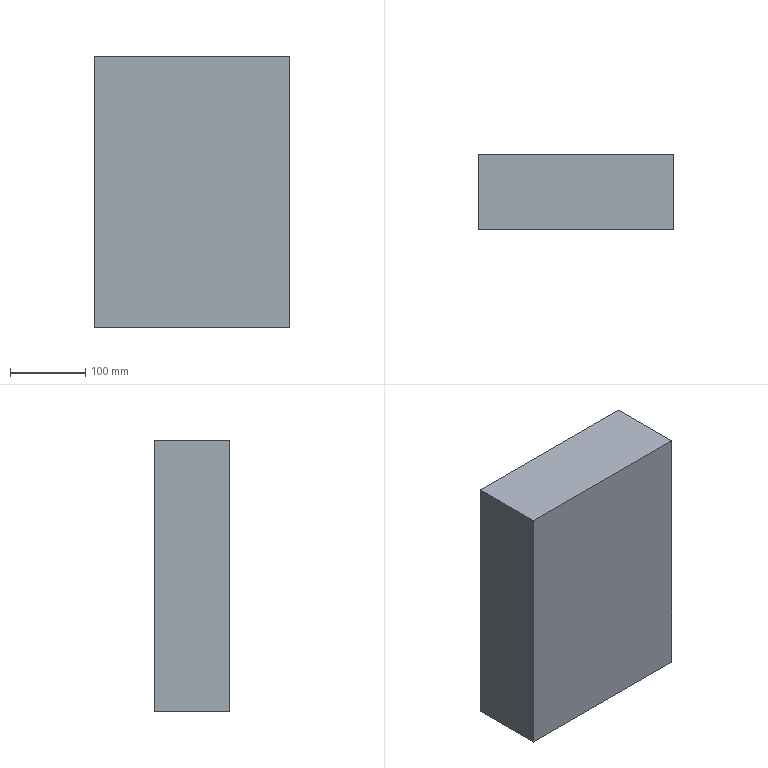Part | STEP file | Part 60 | 1 solid | 1209 faces | box 260 x 100 x 360 mm | volume 9327526 mm3 | plane 1207 | cylinder 2 | commonest cylinder face diameters 30 x2